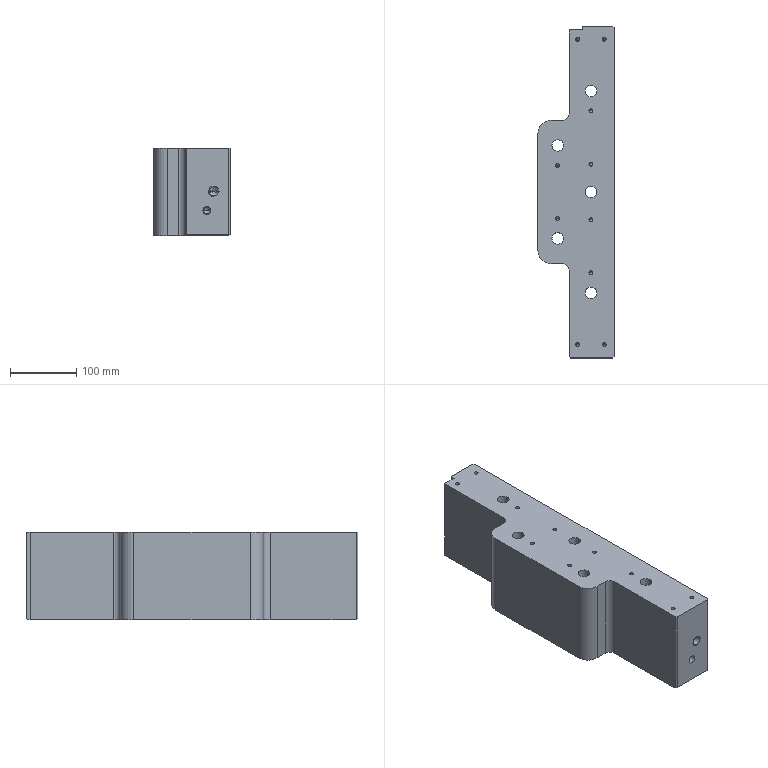Part | Creo | 2 solids | 307 faces | box 115 x 500 x 132 mm | volume 5615538 mm3 | plane 92 | cylinder 78 | other 77 | cone 60 | commonest cylinder face diameters 4.97 x24 6 x24 17.4 x10 10.5 x4 13.9 x4 10.2 x2